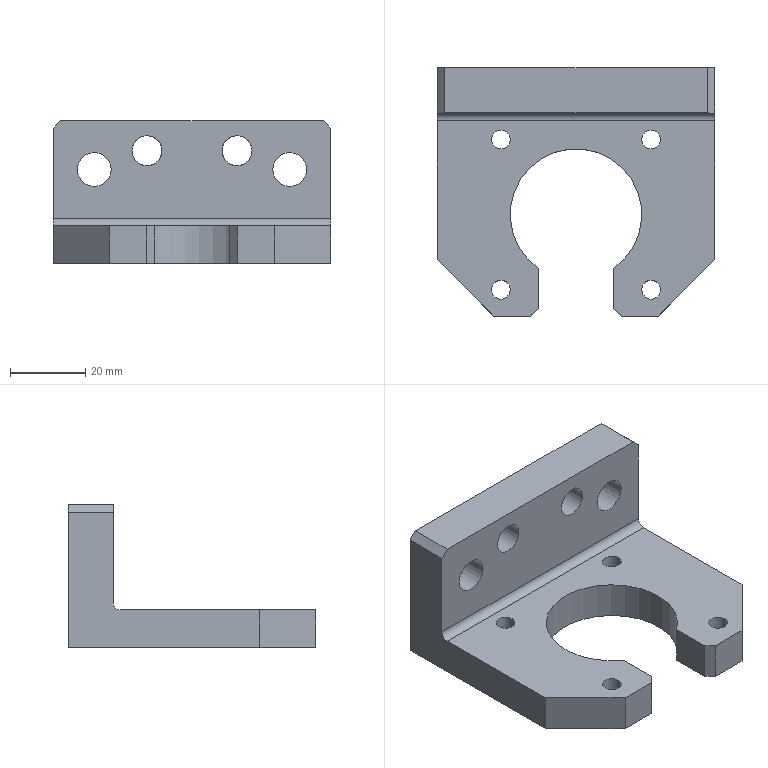Part | STEP file | J454-EBZ05-07-00-Part-1 | 1 solid | 39 faces | box 74 x 66 x 38 mm | volume 56161 mm3 | cylinder 18 | plane 17 | cone 4 | commonest cylinder face diameters 5 x8 8 x4 9 x4 4 x1 35 x1